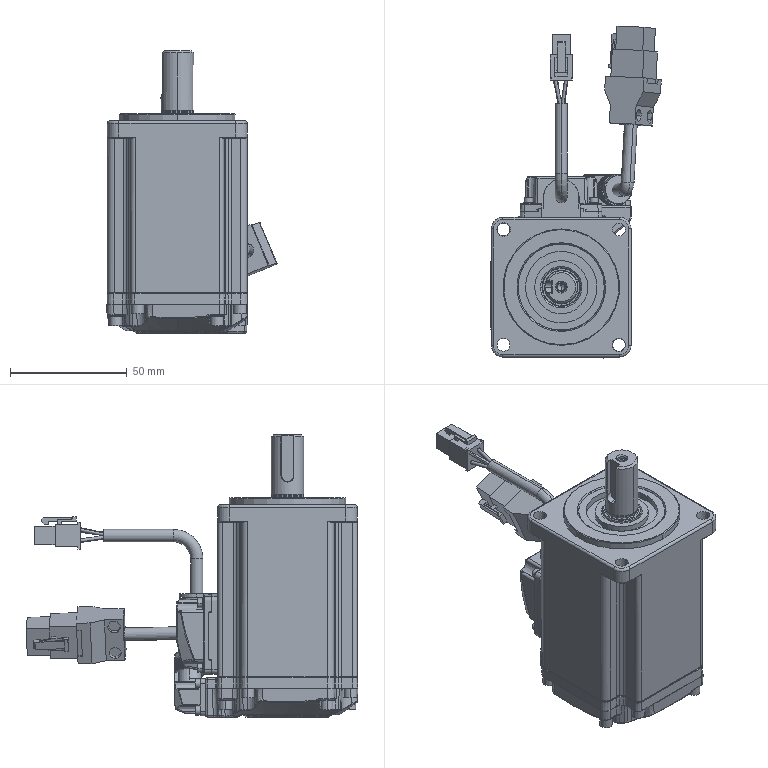Part | 8 solids | 1747 faces | box 73.191 x 142.408 x 121 mm | volume 331662 mm3 | plane 705 | cylinder 550 | cone 185 | spline 153 | torus 126 | sphere 28 | commonest cylinder face diameters 0.4 x134 1 x90 4 x47 2 x39 6 x24 9 x24